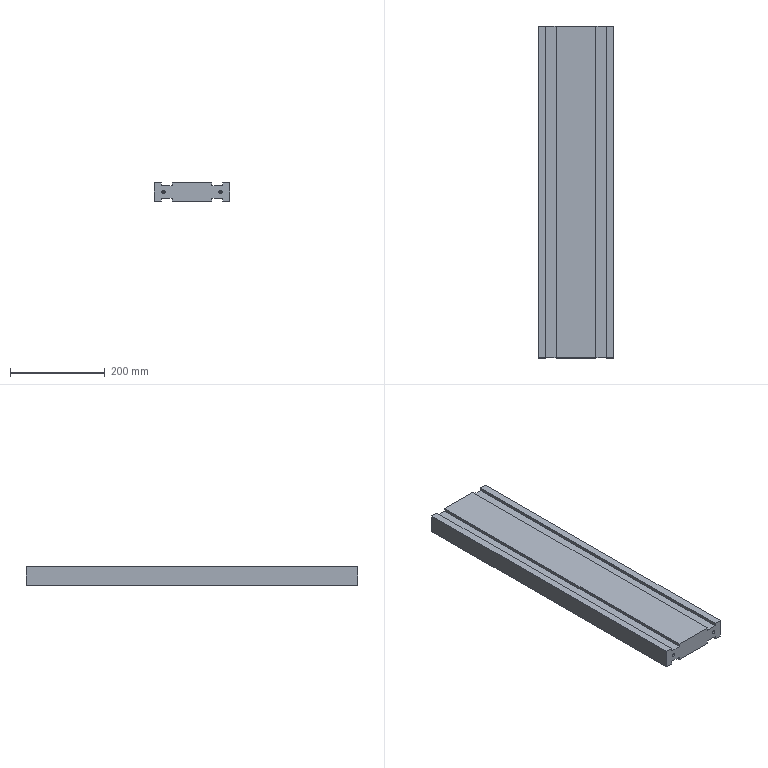Part | 1 solid | 150 faces | box 160 x 700 x 40 mm | volume 4068614 mm3 | cylinder 64 | cone 64 | plane 22 | commonest cylinder face diameters 3.3 x56 6.8 x8